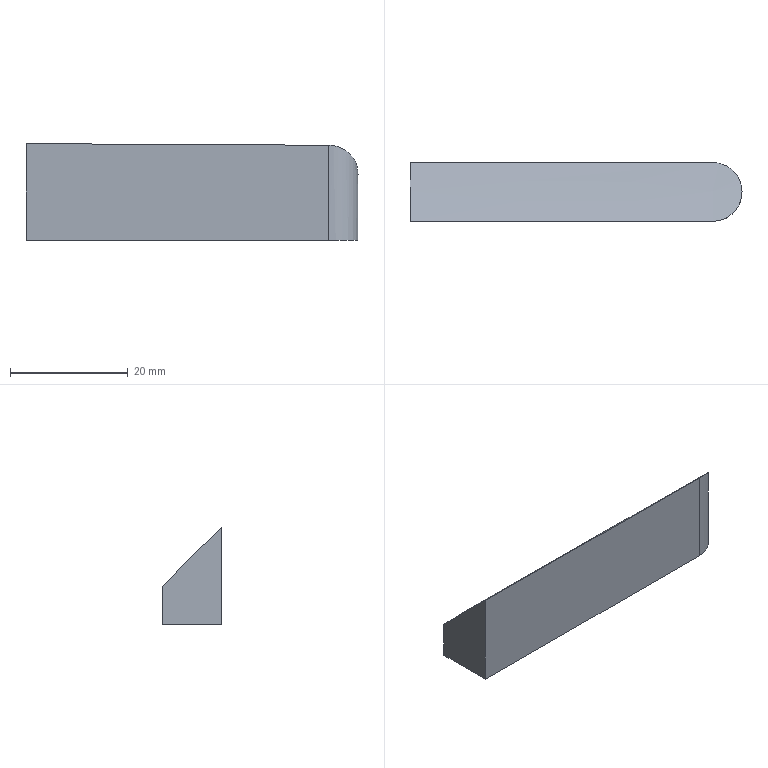Part | NX | features solid 2 | 1 solid | 6 faces | box 56.5 x 10 x 16.452 mm | volume 6331 mm3 | plane 4 | cylinder 1 | spline 1 | commonest cylinder face diameters 10 x1
STEP:
#1=CARTESIAN_POINT('',(71.,712.5,-115.));
#2=VERTEX_POINT('',#1);
#3=CARTESIAN_POINT('',(71.,722.5,-115.));
#4=VERTEX_POINT('',#3);
#5=CARTESIAN_POINT('',(71.,725.,-115.));
#6=DIRECTION('',(0.,-1.,0.));
#7=VECTOR('',#6,1000.);
#8=LINE('',#5,#7);
#9=EDGE_CURVE('',#2,#4,#8,.F.);
#10=ORIENTED_EDGE('',*,*,#9,.F.);
#11=CARTESIAN_POINT('',(71.,712.5,-98.548));
#12=VERTEX_POINT('',#11);
#13=CARTESIAN_POINT('',(71.,712.5,-100.));
#14=DIRECTION('',(0.,0.,1.));
#15=VECTOR('',#14,1000.);
#16=LINE('',#13,#15);
#17=EDGE_CURVE('',#12,#2,#16,.F.);
#18=ORIENTED_EDGE('',*,*,#17,.F.);
#19=CARTESIAN_POINT('',(71.,722.5,-108.598));
#20=VERTEX_POINT('',#19);
#21=CARTESIAN_POINT('',(71.,712.5,-98.548));
#22=CARTESIAN_POINT('',(71.,715.986,-101.744));
#23=CARTESIAN_POINT('',(71.,719.324,-105.099));
#24=CARTESIAN_POINT('',(71.,722.5,-108.598));
#25=B_SPLINE_CURVE_WITH_KNOTS('',3,(#21,#22,#23,#24),.UNSPECIFIED.,.F.,.F.,(4,4),(0.01494,0.02912),.UNSPECIFIED.);
#26=EDGE_CURVE('',#12,#20,#25,.T.);
#27=ORIENTED_EDGE('',*,*,#26,.T.);
#28=CARTESIAN_POINT('',(71.,722.5,-220.));
#29=DIRECTION('',(0.,0.,1.));
#30=VECTOR('',#29,1000.);
#31=LINE('',#28,#30);
#32=EDGE_CURVE('',#20,#4,#31,.F.);
#33=ORIENTED_EDGE('',*,*,#32,.T.);
#34=EDGE_LOOP('',(#10,#18,#27,#33));
#35=FACE_BOUND('',#34,.T.);
#36=CARTESIAN_POINT('',(71.,-448.772,-220.));
#37=DIRECTION('',(-1.,0.,0.));
#38=DIRECTION('',(0.,0.,-1.));
#39=AXIS2_PLACEMENT_3D('',#36,#37,#38);
#40=PLANE('',#39);
#41=ADVANCED_FACE('',(#35),#40,.T.);
#42=CARTESIAN_POINT('',(122.5,722.5,-115.));
#43=VERTEX_POINT('',#42);
#44=CARTESIAN_POINT('',(-10.,722.5,-115.));
#45=DIRECTION('',(-1.,0.,0.));
#46=VECTOR('',#45,1000.);
#47=LINE('',#44,#46);
#48=EDGE_CURVE('',#43,#4,#47,.T.);
#49=ORIENTED_EDGE('',*,*,#48,.T.);
#50=ORIENTED_EDGE('',*,*,#32,.F.);
#51=CARTESIAN_POINT('',(122.5,722.5,-108.957));
#52=VERTEX_POINT('',#51);
#53=CARTESIAN_POINT('',(122.5,722.5,-108.957));
#54=CARTESIAN_POINT('',(105.334,722.5,-108.818));
#55=CARTESIAN_POINT('',(88.167,722.5,-108.699));
#56=CARTESIAN_POINT('',(71.,722.5,-108.598));
#57=B_SPLINE_CURVE_WITH_KNOTS('',3,(#53,#54,#55,#56),.UNSPECIFIED.,.F.,.F.,(4,4),(0.4251,0.4766),.UNSPECIFIED.);
#58=EDGE_CURVE('',#52,#20,#57,.T.);
#59=ORIENTED_EDGE('',*,*,#58,.F.);
#60=CARTESIAN_POINT('',(122.5,722.5,-100.));
#61=DIRECTION('',(0.,0.,-1.));
#62=VECTOR('',#61,1000.);
#63=LINE('',#60,#62);
#64=EDGE_CURVE('',#52,#43,#63,.T.);
#65=ORIENTED_EDGE('',*,*,#64,.T.);
#66=EDGE_LOOP('',(#49,#50,#59,#65));
#67=FACE_BOUND('',#66,.T.);
#68=CARTESIAN_POINT('',(-10.,722.5,-100.));
#69=DIRECTION('',(0.,1.,0.));
#70=DIRECTION('',(0.,0.,1.));
#71=AXIS2_PLACEMENT_3D('',#68,#69,#70);
#72=PLANE('',#71);
#73=ADVANCED_FACE('',(#67),#72,.T.);
#74=CARTESIAN_POINT('',(122.5,712.5,-115.));
#75=VERTEX_POINT('',#74);
#76=CARTESIAN_POINT('',(122.5,717.5,-115.));
#77=DIRECTION('',(0.,0.,1.));
#78=DIRECTION('',(1.,0.,0.));
#79=AXIS2_PLACEMENT_3D('',#76,#77,#78);
#80=CIRCLE('',#79,5.);
#81=EDGE_CURVE('',#75,#43,#80,.T.);
#82=ORIENTED_EDGE('',*,*,#81,.T.);
#83=ORIENTED_EDGE('',*,*,#64,.F.);
#84=CARTESIAN_POINT('',(122.5,712.5,-98.814));
#85=VERTEX_POINT('',#84);
#86=CARTESIAN_POINT('',(122.5,712.5,-98.814));
#87=CARTESIAN_POINT('',(123.3,712.5,-98.819));
#88=CARTESIAN_POINT('',(124.886,712.914,-99.21));
#89=CARTESIAN_POINT('',(127.006,714.73,-100.934));
#90=CARTESIAN_POINT('',(127.854,717.618,-103.775));
#91=CARTESIAN_POINT('',(126.927,720.349,-106.633));
#92=CARTESIAN_POINT('',(124.871,722.086,-108.514));
#93=CARTESIAN_POINT('',(123.303,722.5,-108.964));
#94=CARTESIAN_POINT('',(122.5,722.5,-108.957));
#95=B_SPLINE_CURVE_WITH_KNOTS('',3,(#86,#87,#88,#89,#90,#91,#92,#93,#94),.UNSPECIFIED.,.F.,.F.,(4,1,1,1,1,1,4),(0.03254,0.03492,0.03731,0.04208,0.04685,0.04923,0.05162),.UNSPECIFIED.);
#96=EDGE_CURVE('',#85,#52,#95,.T.);
#97=ORIENTED_EDGE('',*,*,#96,.F.);
#98=CARTESIAN_POINT('',(122.5,712.5,-100.));
#99=DIRECTION('',(0.,0.,-1.));
#100=VECTOR('',#99,1000.);
#101=LINE('',#98,#100);
#102=EDGE_CURVE('',#85,#75,#101,.T.);
#103=ORIENTED_EDGE('',*,*,#102,.T.);
#104=EDGE_LOOP('',(#82,#83,#97,#103));
#105=FACE_BOUND('',#104,.T.);
#106=CARTESIAN_POINT('',(122.5,717.5,-100.));
#107=DIRECTION('',(0.,0.,-1.));
#108=DIRECTION('',(1.,0.,0.));
#109=AXIS2_PLACEMENT_3D('',#106,#107,#108);
#110=CYLINDRICAL_SURFACE('',#109,5.);
#111=ADVANCED_FACE('',(#105),#110,.T.);
#112=CARTESIAN_POINT('',(-10.,712.5,-115.));
#113=DIRECTION('',(1.,0.,0.));
#114=VECTOR('',#113,1000.);
#115=LINE('',#112,#114);
#116=EDGE_CURVE('',#2,#75,#115,.T.);
#117=ORIENTED_EDGE('',*,*,#116,.T.);
#118=ORIENTED_EDGE('',*,*,#102,.F.);
#119=CARTESIAN_POINT('',(71.,712.5,-98.548));
#120=CARTESIAN_POINT('',(88.167,712.5,-98.624));
#121=CARTESIAN_POINT('',(105.333,712.5,-98.712));
#122=CARTESIAN_POINT('',(122.5,712.5,-98.814));
#123=B_SPLINE_CURVE_WITH_KNOTS('',3,(#119,#120,#121,#122),.UNSPECIFIED.,.F.,.F.,(4,4),(0.,0.0515),.UNSPECIFIED.);
#124=EDGE_CURVE('',#12,#85,#123,.T.);
#125=ORIENTED_EDGE('',*,*,#124,.F.);
#126=ORIENTED_EDGE('',*,*,#17,.T.);
#127=EDGE_LOOP('',(#117,#118,#125,#126));
#128=FACE_BOUND('',#127,.T.);
#129=CARTESIAN_POINT('',(-10.,712.5,-100.));
#130=DIRECTION('',(0.,-1.,0.));
#131=DIRECTION('',(0.,0.,-1.));
#132=AXIS2_PLACEMENT_3D('',#129,#130,#131);
#133=PLANE('',#132);
#134=ADVANCED_FACE('',(#128),#133,.T.);
#135=ORIENTED_EDGE('',*,*,#26,.F.);
#136=ORIENTED_EDGE('',*,*,#124,.T.);
#137=ORIENTED_EDGE('',*,*,#96,.T.);
#138=ORIENTED_EDGE('',*,*,#58,.T.);
#139=EDGE_LOOP('',(#135,#136,#137,#138));
#140=FACE_BOUND('',#139,.T.);
#141=CARTESIAN_POINT('',(70.661,712.437,-98.49));
#142=CARTESIAN_POINT('',(70.653,716.014,-101.764));
#143=CARTESIAN_POINT('',(70.646,719.431,-105.203));
#144=CARTESIAN_POINT('',(70.639,722.691,-108.807));
#145=CARTESIAN_POINT('',(89.747,712.39,-98.53));
#146=CARTESIAN_POINT('',(89.733,715.974,-101.819));
#147=CARTESIAN_POINT('',(89.72,719.399,-105.272));
#148=CARTESIAN_POINT('',(89.707,722.665,-108.89));
#149=CARTESIAN_POINT('',(108.833,712.323,-98.567));
#150=CARTESIAN_POINT('',(108.814,715.912,-101.87));
#151=CARTESIAN_POINT('',(108.795,719.342,-105.337));
#152=CARTESIAN_POINT('',(108.776,722.614,-108.969));
#153=CARTESIAN_POINT('',(127.92,712.235,-98.602));
#154=CARTESIAN_POINT('',(127.894,715.828,-101.918));
#155=CARTESIAN_POINT('',(127.869,719.262,-105.398));
#156=CARTESIAN_POINT('',(127.844,722.538,-109.043));
#157=B_SPLINE_SURFACE_WITH_KNOTS('',3,3,((#141,#142,#143,#144),(#145,#146,#147,#148),(#149,#150,#151,#152),(#153,#154,#155,#156)),.UNSPECIFIED.,.F.,.F.,.F.,(4,4),(4,4),(-0.003661,0.08163),(0.4868,0.7262),.UNSPECIFIED.);
#158=ADVANCED_FACE('',(#140),#157,.T.);
#159=ORIENTED_EDGE('',*,*,#9,.T.);
#160=ORIENTED_EDGE('',*,*,#48,.F.);
#161=ORIENTED_EDGE('',*,*,#81,.F.);
#162=ORIENTED_EDGE('',*,*,#116,.F.);
#163=EDGE_LOOP('',(#159,#160,#161,#162));
#164=FACE_BOUND('',#163,.T.);
#165=CARTESIAN_POINT('',(-10.,725.,-115.));
#166=DIRECTION('',(0.,0.,-1.));
#167=DIRECTION('',(1.,0.,0.));
#168=AXIS2_PLACEMENT_3D('',#165,#166,#167);
#169=PLANE('',#168);
#170=ADVANCED_FACE('',(#164),#169,.T.);
#171=CLOSED_SHELL('',(#41,#73,#111,#134,#158,#170));
#172=MANIFOLD_SOLID_BREP('',#171);
#173=(LENGTH_UNIT()NAMED_UNIT(*)SI_UNIT(.MILLI.,.METRE.));
#174=UNCERTAINTY_MEASURE_WITH_UNIT(LENGTH_MEASURE(0.0508),#173,'','');
#175=(NAMED_UNIT(*)PLANE_ANGLE_UNIT()SI_UNIT($,.RADIAN.));
#176=(NAMED_UNIT(*)SI_UNIT($,.STERADIAN.)SOLID_ANGLE_UNIT());
#177=(GEOMETRIC_REPRESENTATION_CONTEXT(3)GLOBAL_UNCERTAINTY_ASSIGNED_CONTEXT((#174))GLOBAL_UNIT_ASSIGNED_CONTEXT((#173,#175,#176))REPRESENTATION_CONTEXT('',''));
#178=ADVANCED_BREP_SHAPE_REPRESENTATION('',(#172),#177);